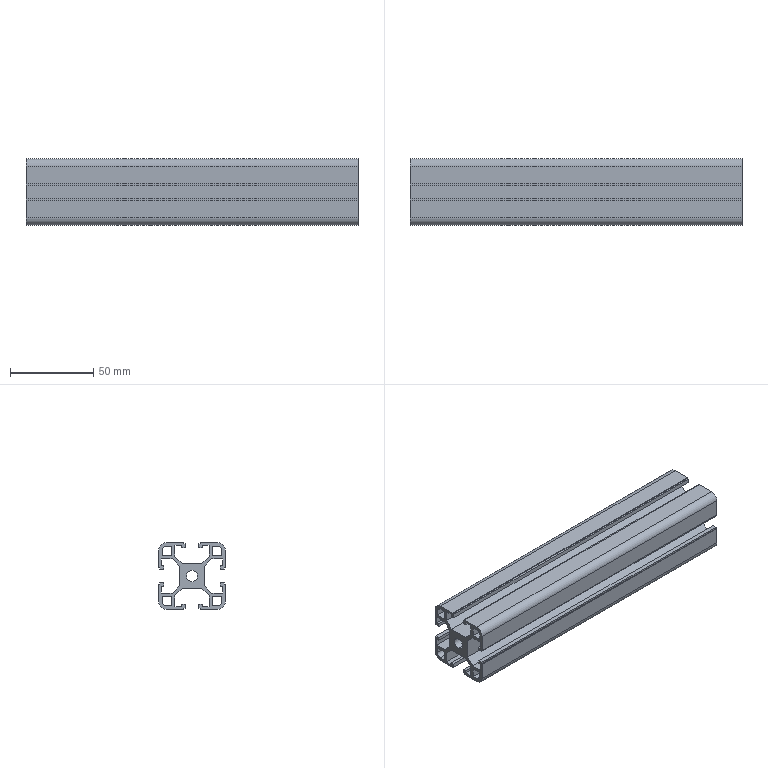Part | SolidWorks | features WeldMemberFeat 1, WeldmentFeature 1 | 1 solid | 104 faces | box 200 x 40 x 40 mm | volume 115309 mm3 | plane 94 | cylinder 10 | commonest cylinder face diameters 5 x4 9 x4 6.8 x2